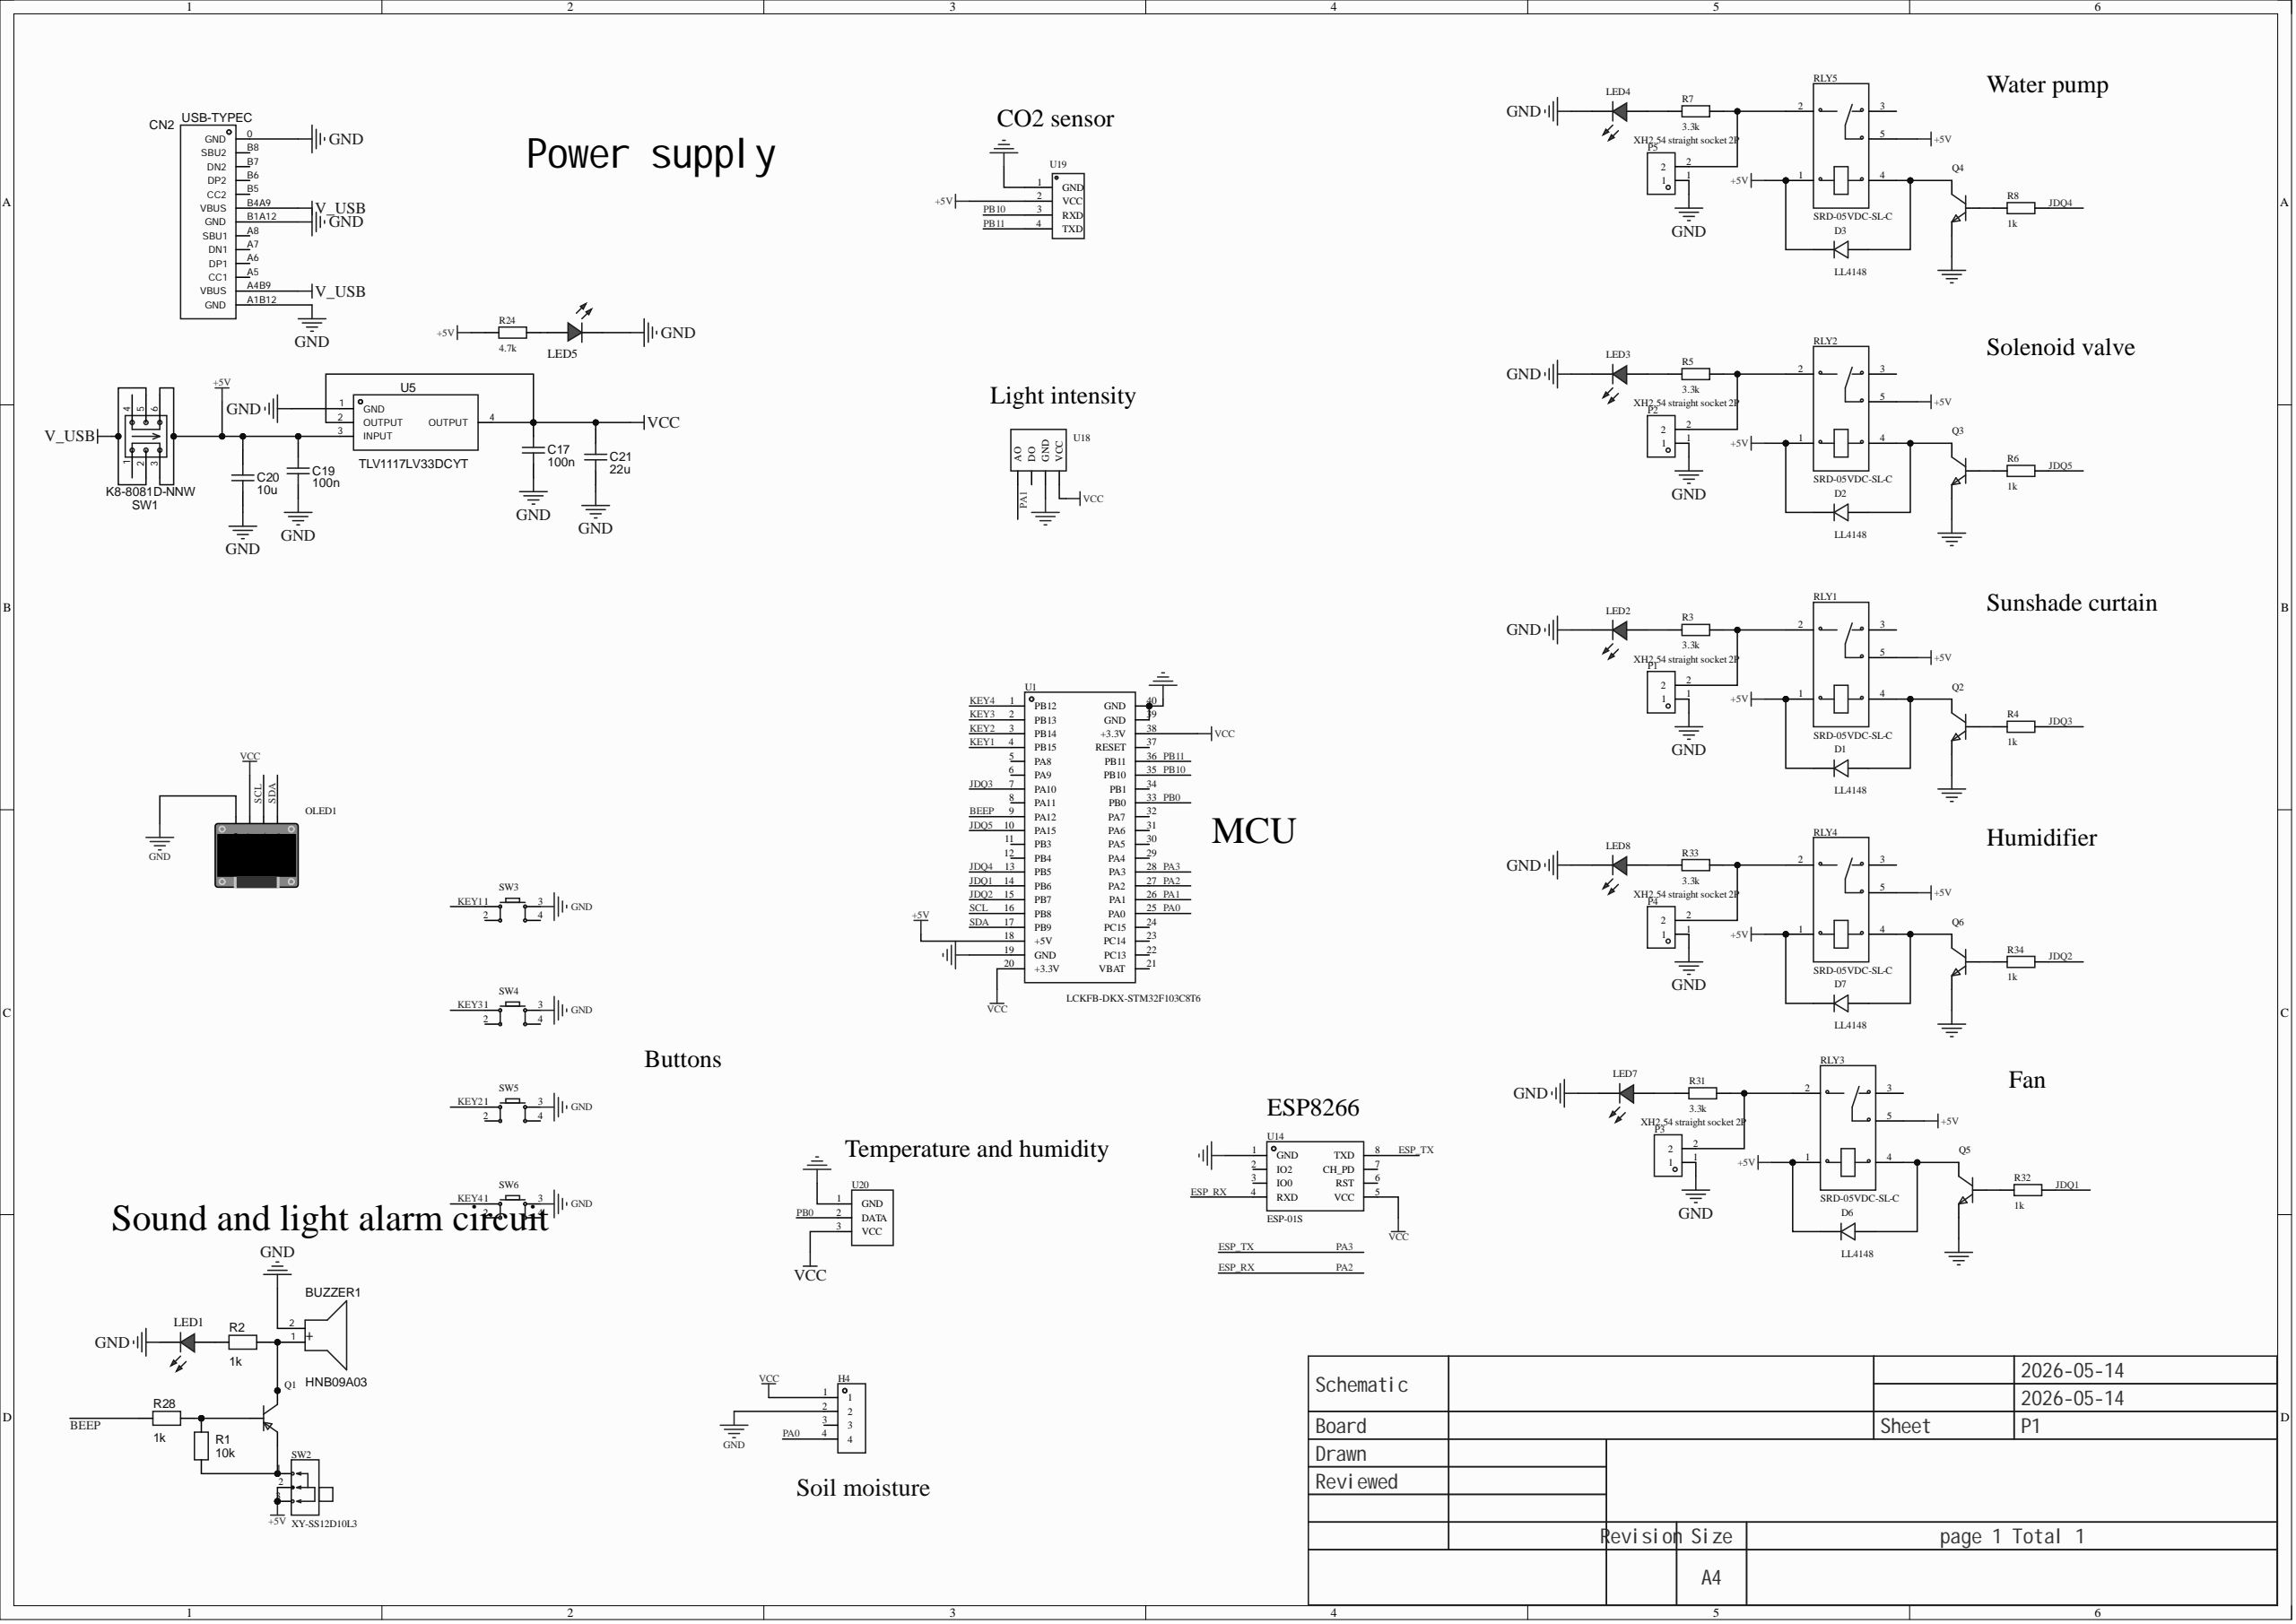Circuit board | Altium Designer | 62 parts | 48 nets
Bill of materials:
Comment,Description,Designator,Footprint,LibRef,Quantity
"HNB09A03","","BUZZER1","BUZ-TH_BD9.0-P5.00-D0.6-FD","HNB09A03","1"
"100n","","C17, C19","C0603","100n","2"
"10u","","C20","C0603","100n","1"
"22u","","C21","C0603","100n","1"
"USB-TYPEC","","CN2","USB-C-SMD_MC-307","MC-307","1"
"LL4148","Diode configuration: -; power: 500mW; DC reverse withstand voltage (Vr): 75V; average rectified current (Io): 200mA; forward voltage (Vf): 1V@10mA; reverse current (Ir): 5uA@75V; reverse recovery time (trr): 4ns; operating temperature: +175℃@(Tj);","D1, D2, D3, D6, D7","LL-34_L3.5-W1.5-RD","LL4148_C9808","5"
"","","H4","HDR-TH_4P-P2.54-V-F","HDR-F_2.54_1x4P","1"
"","","LED1, LED5","LED_0603","LED_0603-R","2"
"","","LED2, LED3, LED4, LED7, LED8","LED_TH-3mm","LED_TH-R_3mm","5"
"","","OLED1","0.96OLED_4P","0.96OLED模块_4P","1"
"XH2.54 straight socket 2P","","P1, P2, P3, P4, P5","CONN-TH_XH2.54-2P","XH2.54直插座-2P","5"
"","","Q1","S8550P_SOT","S8550_SOT_PNP","1"
"","","Q2, Q3, Q4, Q5, Q6","S8050_SOT-23","S8050_SOT_NPN","5"
"10k","","R1","R0603","1k","1"
"1k","","R2, R4, R6, R8, R28, R32, R34","R0603","1k, Res_0603","7"
"3.3k","","R3, R5, R7, R31, R33","R0603","Res_0603","5"
"4.7k","Resistor type: thick film resistor; resistance: 10kO; tolerance: ±1%; power: 125mW;","R24","R0805","0805W8F1002T5E_C17414","1"
"SRD-05VDC-SL-C","Coil voltage: 5V; contact form: 1C (SPDT changeover); contact rating (resistive load): -; max switching voltage: 250V@AC; max switching current: 15A;","RLY1, RLY2, RLY3, RLY4, RLY5","RELAY-TH_SRD-XXVDC-XL-C","SRD-05VDC-SL-C","5"
"K8-8081D-NNW","","SW1","SW-TH_6P-L8.0-W8.0-P2.50","XKB8080-Z","1"
"XY-SS12D10L3","Toggle switch, vertical straight pins, two-position, through-hole, single row, forward actuation, lever length 3mm","SW2","SW-TH_3P-L12.7-W6.7_XY-SS12D10LXX","XY-SS12D10L3","1"
"","","SW3, SW4, SW5, SW6","SW-TH_4P-L6.0-W6.0-P4.50-LS6.5","Key_TH_6x6x6","4"
"LCKFB-DKX-STM32F103C8T6","","U1","CONN-TH_L53.3-W22.9_STM32F103C8T6-CARD","LCKFB-DKX-STM32F103C8T6","1"
"TLV1117LV33DCYT","","U5","SOT-223-4_L6.5-W3.5-P2.30-LS7.0-BR","TLV1117LV33DCYT","1"
"ESP-01S","","U14","WIFIM-TH_ESP-01S","ESP-01S_C111009","1"
"Light intensity module","","U18","光敏传感器","光照强度模块","1"
"","","U19","4P排母","二氧化碳传感器","1"
"","","U20","dht11温湿度传感器","DHT11","1"
Netlist (Protel format):
[
BUZZER1
BUZ-TH_BD9.0-P5.00-D0.6-FD
HNB09A03



]
[
C17
C0603
100n



]
[
C19
C0603
100n



]
[
C20
C0603
10u



]
[
C21
C0603
22u



]
[
CN2
USB-C-SMD_MC-307
USB-TYPEC



]
[
D1
LL-34_L3.5-W1.5-RD
LL4148



]
[
D2
LL-34_L3.5-W1.5-RD
LL4148



]
[
D3
LL-34_L3.5-W1.5-RD
LL4148



]
[
D6
LL-34_L3.5-W1.5-RD
LL4148



]
[
D7
LL-34_L3.5-W1.5-RD
LL4148



]
[
H4
HDR-TH_4P-P2.54-V-F




]
[
LED1
LED_0603




]
[
LED2
LED_TH-3mm




]
[
LED3
LED_TH-3mm




]
[
LED4
LED_TH-3mm




]
[
LED5
LED_0603




]
[
LED7
LED_TH-3mm




]
[
LED8
LED_TH-3mm




]
[
OLED1
0.96OLED_4P




]
[
P1
CONN-TH_XH2.54-2P
XH2.54 straight socket 2P



]
[
P2
CONN-TH_XH2.54-2P
XH2.54 straight socket 2P



]
[
P3
CONN-TH_XH2.54-2P
XH2.54 straight socket 2P



]
[
P4
CONN-TH_XH2.54-2P
XH2.54 straight socket 2P



]
[
P5
CONN-TH_XH2.54-2P
XH2.54 straight socket 2P



]
[
Q1
S8550P_SOT




]
[
Q2
S8050_SOT-23




]
[
Q3
S8050_SOT-23




]
[
Q4
S8050_SOT-23




]
[
Q5
S8050_SOT-23




]
[
Q6
S8050_SOT-23




]
[
R1
R0603
10k



]
[
R2
R0603
1k



]
[
R3
R0603
3.3k



]
[
R4
R0603
1k



]
[
R5
R0603
3.3k



]
[
R6
R0603
1k



]
[
R7
R0603
3.3k



]
[
R8
R0603
1k



]
[
R24
R0805
4.7k



]
[
R28
R0603
1k



]
[
R31
R0603
3.3k



]
[
R32
R0603
1k



]
[
R33
R0603
3.3k



]
[
R34
R0603
1k



]
[
RLY1
RELAY-TH_SRD-XXVDC-XL-C
SRD-05VDC-SL-C



]
[
RLY2
RELAY-TH_SRD-XXVDC-XL-C
SRD-05VDC-SL-C



]
[
RLY3
RELAY-TH_SRD-XXVDC-XL-C
SRD-05VDC-SL-C



]
[
RLY4
RELAY-TH_SRD-XXVDC-XL-C
SRD-05VDC-SL-C



]
[
RLY5
RELAY-TH_SRD-XXVDC-XL-C
SRD-05VDC-SL-C



]
[
SW1
SW-TH_6P-L8.0-W8.0-P2.50
K8-8081D-NNW



]
[
SW2
SW-TH_3P-L12.7-W6.7_XY-SS12D10LXX
XY-SS12D10L3



]
[
SW3
SW-TH_4P-L6.0-W6.0-P4.50-LS6.5




]
[
SW4
SW-TH_4P-L6.0-W6.0-P4.50-LS6.5




]
[
SW5
SW-TH_4P-L6.0-W6.0-P4.50-LS6.5




]
[
SW6
SW-TH_4P-L6.0-W6.0-P4.50-LS6.5




]
[
U1
CONN-TH_L53.3-W22.9_STM32F103C8T6-CARD
LCKFB-DKX-STM32F103C8T6



]
[
U5
SOT-223-4_L6.5-W3.5-P2.30-LS7.0-BR
TLV1117LV33DCYT



]
[
U14
WIFIM-TH_ESP-01S
ESP-01S



]
[
U18
光敏传感器
Light intensity module



]
[
U19
4P排母




]
[
U20
dht11温湿度传感器




]
(
VCC
C17-2
C21-2
H4-1
OLED1-2
U1-20
U1-38
U5-2
U5-4
U14-5
U18-1
U20-3
)
(
V_USB
CN2-A4B9
CN2-B4A9
SW1-2
SW1-5
)
(
SDA
OLED1-4
U1-17
)
(
SCL
OLED1-3
U1-16
)
(
PB11
U1-36
U19-4
)
(
PB10
U1-35
U19-3
)
(
PB0
U1-33
U20-2
)
(
PA1
U1-26
U18-4
)
(
PA0
H4-4
U1-25
)
(
NetQ6_1
Q6-1
R34-2
)
(
NetQ5_1
Q5-1
R32-2
)
(
NetQ4_1
Q4-1
R8-2
)
(
NetQ3_1
Q3-1
R6-2
)
(
NetQ2_1
Q2-1
R4-2
)
(
NetQ1_2
Q1-2
R1-1
SW2-1
)
(
NetQ1_1
Q1-1
R1-2
R28-2
)
(
NetP5_2
P5-2
R7-1
RLY5-2
)
(
NetP4_2
P4-2
R33-1
RLY4-2
)
(
NetP3_2
P3-2
R31-1
RLY3-2
)
(
NetP2_2
P2-2
R5-1
RLY2-2
)
(
NetP1_2
P1-2
R3-1
RLY1-2
)
(
NetLED8_1
LED8-1
R33-2
)
(
NetLED7_1
LED7-1
R31-2
)
(
NetLED5_2
LED5-2
R24-2
)
(
NetLED4_1
LED4-1
R7-2
)
(
NetLED3_1
LED3-1
R5-2
)
(
NetLED2_1
LED2-1
R3-2
)
(
NetLED1_2
LED1-2
R2-1
)
(
NetD7_2
D7-2
Q6-3
RLY4-4
)
(
NetD6_2
D6-2
Q5-3
RLY3-4
)
(
NetD3_2
D3-2
Q4-3
RLY5-4
)
(
NetD2_2
D2-2
Q3-3
RLY2-4
)
(
NetD1_2
D1-2
Q2-3
RLY1-4
)
(
NetBUZZER1_1
BUZZER1-1
Q1-3
R2-2
)
(
KEY4
SW6-1
U1-1
)
(
KEY3
SW4-1
U1-2
)
(
KEY2
SW5-1
U1-3
)
(
KEY1
SW3-1
U1-4
)
(
JDQ5
R6-1
U1-10
)
(
JDQ4
R8-1
U1-13
)
(
JDQ3
R4-1
U1-7
)
(
JDQ2
R34-1
U1-15
)
(
JDQ1
R32-1
U1-14
)
(
GND
BUZZER1-2
C17-1
C19-1
C20-1
C21-1
CN2-0
CN2-A1B12
CN2-B1A12
H4-2
LED1-1
LED2-2
LED3-2
LED4-2
LED5-1
LED7-2
LED8-2
OLED1-1
P1-1
P2-1
P3-1
P4-1
P5-1
Q2-2
Q3-2
Q4-2
Q5-2
Q6-2
SW3-3
SW4-3
SW5-3
SW6-3
U1-19
U1-39
U1-40
U5-1
U14-1
U18-2
U19-1
U20-1
)
(
ESP_TX
U1-28
U14-8
)
(
ESP_RX
U1-27
U14-4
)
(
BEEP
R28-1
U1-9
)
(
+5V
C19-2
C20-2
D1-1
D2-1
D3-1
D6-1
D7-1
R24-1
RLY1-1
RLY1-5
RLY2-1
RLY2-5
RLY3-1
RLY3-5
RLY4-1
RLY4-5
RLY5-1
RLY5-5
SW1-3
SW1-6
SW2-2
SW2-3
U1-18
U5-3
U19-2
)